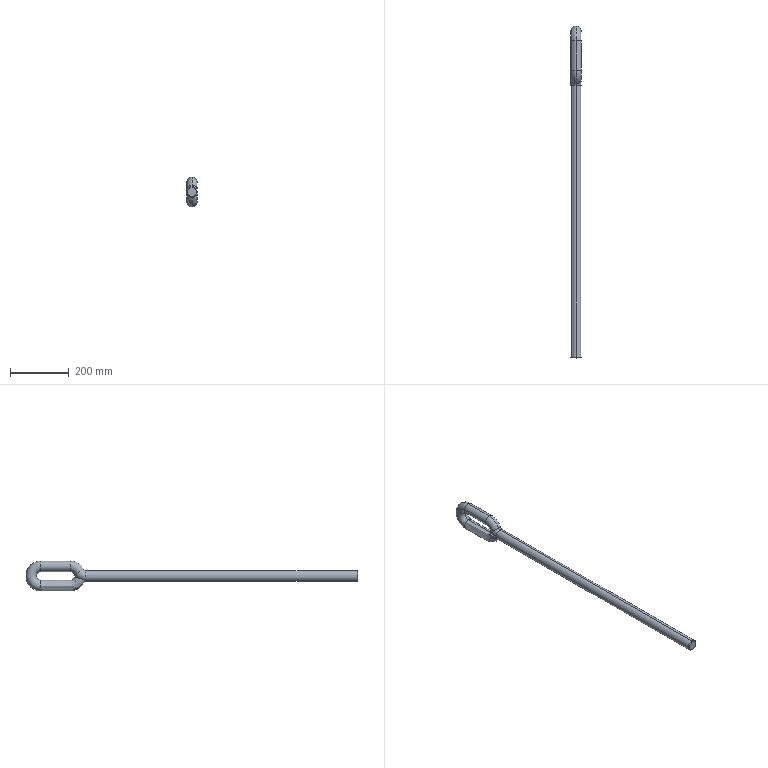Part | SolidWorks | features Chamfer 1, Sweep 1 | 1 solid | 16 faces | box 36 x 1131 x 102 mm | volume 1361962 mm3 | torus 6 | cylinder 4 | cone 2 | spline 2 | plane 2 | commonest cylinder face diameters 36 x4